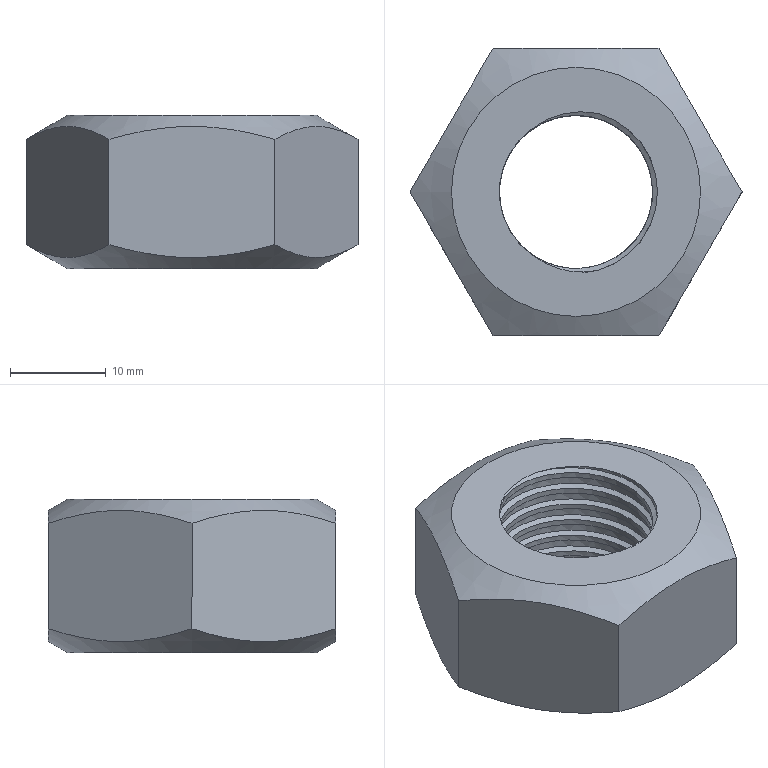Part | NX | features DATUM_CSYS 3, SKETCH 2, EXTRUDE 1, SWP104 1, THREADS 1 | 1 solid | 15 faces | box 34.641 x 30 x 16 mm | volume 8595 mm3 | plane 9 | cylinder 2 | spline 2 | cone 2 | commonest cylinder face diameters 16 x1 17 x1